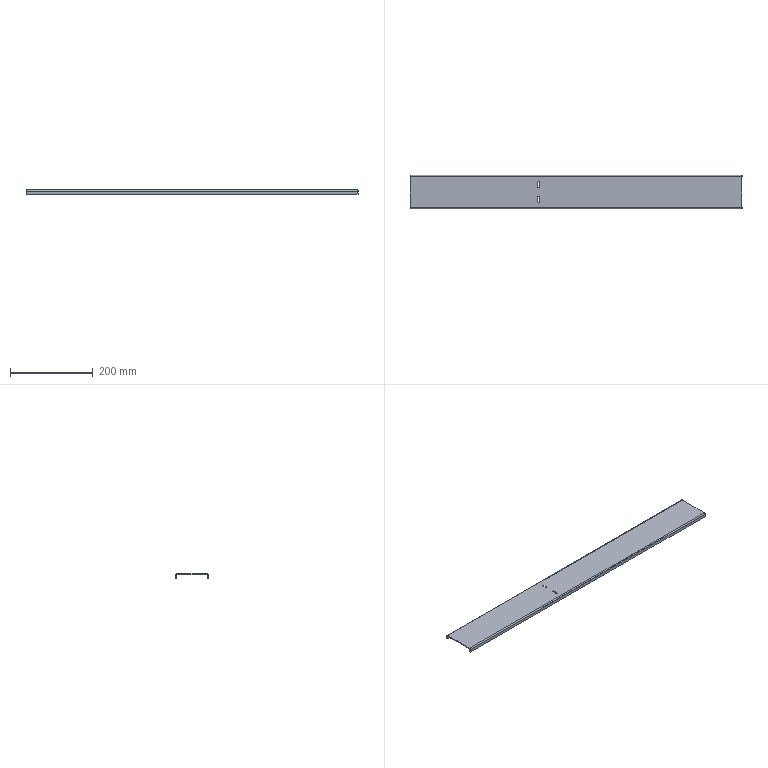Part | SolidWorks | features EdgeFlange 1, FlatPattern 1, ICE 1, SMBaseFlange 1, SheetMetal 1 | 1 solid | 30 faces | box 800 x 80 x 10 mm | volume 150971 mm3 | plane 22 | cylinder 8 | commonest cylinder face diameters 4.5 x4 1.473 x2 5.473 x2
STEP:
#1=CARTESIAN_POINT('',(-87.75,-12.5,-2.));
#2=VERTEX_POINT('',#1);
#3=CARTESIAN_POINT('',(-87.75,-22.5,-2.));
#4=VERTEX_POINT('',#3);
#5=CARTESIAN_POINT('',(-87.75,-12.5,-2.));
#6=DIRECTION('',(0.,-1.,0.));
#7=VECTOR('',#6,1000.);
#8=LINE('',#5,#7);
#9=EDGE_CURVE('',#2,#4,#8,.T.);
#10=ORIENTED_EDGE('',*,*,#9,.F.);
#11=CARTESIAN_POINT('',(-92.25,-12.5,-2.));
#12=VERTEX_POINT('',#11);
#13=CARTESIAN_POINT('',(-90.,-12.5,-2.));
#14=DIRECTION('',(0.,0.,-1.));
#15=DIRECTION('',(-1.,0.,0.));
#16=AXIS2_PLACEMENT_3D('',#13,#14,#15);
#17=CIRCLE('',#16,2.25);
#18=EDGE_CURVE('',#12,#2,#17,.T.);
#19=ORIENTED_EDGE('',*,*,#18,.F.);
#20=CARTESIAN_POINT('',(-92.25,-22.5,-2.));
#21=VERTEX_POINT('',#20);
#22=CARTESIAN_POINT('',(-92.25,-12.5,-2.));
#23=DIRECTION('',(0.,1.,0.));
#24=VECTOR('',#23,1000.);
#25=LINE('',#22,#24);
#26=EDGE_CURVE('',#21,#12,#25,.T.);
#27=ORIENTED_EDGE('',*,*,#26,.F.);
#28=CARTESIAN_POINT('',(-90.,-22.5,-2.));
#29=DIRECTION('',(0.,0.,-1.));
#30=DIRECTION('',(-1.,0.,0.));
#31=AXIS2_PLACEMENT_3D('',#28,#29,#30);
#32=CIRCLE('',#31,2.25);
#33=EDGE_CURVE('',#4,#21,#32,.T.);
#34=ORIENTED_EDGE('',*,*,#33,.F.);
#35=EDGE_LOOP('',(#10,#19,#27,#34));
#36=FACE_BOUND('',#35,.T.);
#37=CARTESIAN_POINT('',(-87.75,22.5,-2.));
#38=VERTEX_POINT('',#37);
#39=CARTESIAN_POINT('',(-87.75,12.5,-2.));
#40=VERTEX_POINT('',#39);
#41=CARTESIAN_POINT('',(-87.75,22.5,-2.));
#42=DIRECTION('',(0.,-1.,0.));
#43=VECTOR('',#42,1000.);
#44=LINE('',#41,#43);
#45=EDGE_CURVE('',#38,#40,#44,.T.);
#46=ORIENTED_EDGE('',*,*,#45,.F.);
#47=CARTESIAN_POINT('',(-92.25,22.5,-2.));
#48=VERTEX_POINT('',#47);
#49=CARTESIAN_POINT('',(-90.,22.5,-2.));
#50=DIRECTION('',(0.,0.,-1.));
#51=DIRECTION('',(-1.,0.,0.));
#52=AXIS2_PLACEMENT_3D('',#49,#50,#51);
#53=CIRCLE('',#52,2.25);
#54=EDGE_CURVE('',#48,#38,#53,.T.);
#55=ORIENTED_EDGE('',*,*,#54,.F.);
#56=CARTESIAN_POINT('',(-92.25,12.5,-2.));
#57=VERTEX_POINT('',#56);
#58=CARTESIAN_POINT('',(-92.25,22.5,-2.));
#59=DIRECTION('',(0.,1.,0.));
#60=VECTOR('',#59,1000.);
#61=LINE('',#58,#60);
#62=EDGE_CURVE('',#57,#48,#61,.T.);
#63=ORIENTED_EDGE('',*,*,#62,.F.);
#64=CARTESIAN_POINT('',(-90.,12.5,-2.));
#65=DIRECTION('',(0.,0.,-1.));
#66=DIRECTION('',(-1.,0.,0.));
#67=AXIS2_PLACEMENT_3D('',#64,#65,#66);
#68=CIRCLE('',#67,2.25);
#69=EDGE_CURVE('',#40,#57,#68,.T.);
#70=ORIENTED_EDGE('',*,*,#69,.F.);
#71=EDGE_LOOP('',(#46,#55,#63,#70));
#72=FACE_BOUND('',#71,.T.);
#73=CARTESIAN_POINT('',(-400.,-37.263,-2.));
#74=VERTEX_POINT('',#73);
#75=CARTESIAN_POINT('',(400.,-37.263,-2.));
#76=VERTEX_POINT('',#75);
#77=CARTESIAN_POINT('',(-400.,-37.263,-2.));
#78=DIRECTION('',(1.,0.,0.));
#79=VECTOR('',#78,1000.);
#80=LINE('',#77,#79);
#81=EDGE_CURVE('',#74,#76,#80,.T.);
#82=ORIENTED_EDGE('',*,*,#81,.F.);
#83=CARTESIAN_POINT('',(-400.,37.263,-2.));
#84=VERTEX_POINT('',#83);
#85=CARTESIAN_POINT('',(-400.,40.,-2.));
#86=DIRECTION('',(0.,-1.,0.));
#87=VECTOR('',#86,1000.);
#88=LINE('',#85,#87);
#89=EDGE_CURVE('',#84,#74,#88,.T.);
#90=ORIENTED_EDGE('',*,*,#89,.F.);
#91=CARTESIAN_POINT('',(400.,37.263,-2.));
#92=VERTEX_POINT('',#91);
#93=CARTESIAN_POINT('',(400.,37.263,-2.));
#94=DIRECTION('',(-1.,0.,0.));
#95=VECTOR('',#94,1000.);
#96=LINE('',#93,#95);
#97=EDGE_CURVE('',#92,#84,#96,.T.);
#98=ORIENTED_EDGE('',*,*,#97,.F.);
#99=CARTESIAN_POINT('',(400.,40.,-2.));
#100=DIRECTION('',(0.,1.,0.));
#101=VECTOR('',#100,1000.);
#102=LINE('',#99,#101);
#103=EDGE_CURVE('',#76,#92,#102,.T.);
#104=ORIENTED_EDGE('',*,*,#103,.F.);
#105=EDGE_LOOP('',(#82,#90,#98,#104));
#106=FACE_OUTER_BOUND('',#105,.T.);
#107=CARTESIAN_POINT('',(0.,0.,-2.));
#108=DIRECTION('',(0.,0.,1.));
#109=DIRECTION('',(1.,0.,0.));
#110=AXIS2_PLACEMENT_3D('',#107,#108,#109);
#111=PLANE('',#110);
#112=ADVANCED_FACE('',(#36,#72,#106),#111,.F.);
#113=CARTESIAN_POINT('',(-87.75,-12.5,0.));
#114=VERTEX_POINT('',#113);
#115=CARTESIAN_POINT('',(-92.25,-12.5,0.));
#116=VERTEX_POINT('',#115);
#117=CARTESIAN_POINT('',(-90.,-12.5,0.));
#118=DIRECTION('',(0.,0.,1.));
#119=DIRECTION('',(1.,0.,0.));
#120=AXIS2_PLACEMENT_3D('',#117,#118,#119);
#121=CIRCLE('',#120,2.25);
#122=EDGE_CURVE('',#114,#116,#121,.T.);
#123=ORIENTED_EDGE('',*,*,#122,.F.);
#124=CARTESIAN_POINT('',(-87.75,-22.5,0.));
#125=VERTEX_POINT('',#124);
#126=CARTESIAN_POINT('',(-87.75,0.,0.));
#127=DIRECTION('',(0.,1.,0.));
#128=VECTOR('',#127,1000.);
#129=LINE('',#126,#128);
#130=EDGE_CURVE('',#125,#114,#129,.T.);
#131=ORIENTED_EDGE('',*,*,#130,.F.);
#132=CARTESIAN_POINT('',(-92.25,-22.5,0.));
#133=VERTEX_POINT('',#132);
#134=CARTESIAN_POINT('',(-90.,-22.5,0.));
#135=DIRECTION('',(0.,0.,1.));
#136=DIRECTION('',(1.,0.,0.));
#137=AXIS2_PLACEMENT_3D('',#134,#135,#136);
#138=CIRCLE('',#137,2.25);
#139=EDGE_CURVE('',#133,#125,#138,.T.);
#140=ORIENTED_EDGE('',*,*,#139,.F.);
#141=CARTESIAN_POINT('',(-92.25,0.,0.));
#142=DIRECTION('',(0.,-1.,0.));
#143=VECTOR('',#142,1000.);
#144=LINE('',#141,#143);
#145=EDGE_CURVE('',#116,#133,#144,.T.);
#146=ORIENTED_EDGE('',*,*,#145,.F.);
#147=EDGE_LOOP('',(#123,#131,#140,#146));
#148=FACE_BOUND('',#147,.T.);
#149=CARTESIAN_POINT('',(-87.75,22.5,0.));
#150=VERTEX_POINT('',#149);
#151=CARTESIAN_POINT('',(-92.25,22.5,0.));
#152=VERTEX_POINT('',#151);
#153=CARTESIAN_POINT('',(-90.,22.5,0.));
#154=DIRECTION('',(0.,0.,1.));
#155=DIRECTION('',(1.,0.,0.));
#156=AXIS2_PLACEMENT_3D('',#153,#154,#155);
#157=CIRCLE('',#156,2.25);
#158=EDGE_CURVE('',#150,#152,#157,.T.);
#159=ORIENTED_EDGE('',*,*,#158,.F.);
#160=CARTESIAN_POINT('',(-87.75,12.5,0.));
#161=VERTEX_POINT('',#160);
#162=CARTESIAN_POINT('',(-87.75,0.,0.));
#163=DIRECTION('',(0.,1.,0.));
#164=VECTOR('',#163,1000.);
#165=LINE('',#162,#164);
#166=EDGE_CURVE('',#161,#150,#165,.T.);
#167=ORIENTED_EDGE('',*,*,#166,.F.);
#168=CARTESIAN_POINT('',(-92.25,12.5,0.));
#169=VERTEX_POINT('',#168);
#170=CARTESIAN_POINT('',(-90.,12.5,0.));
#171=DIRECTION('',(0.,0.,1.));
#172=DIRECTION('',(1.,0.,0.));
#173=AXIS2_PLACEMENT_3D('',#170,#171,#172);
#174=CIRCLE('',#173,2.25);
#175=EDGE_CURVE('',#169,#161,#174,.T.);
#176=ORIENTED_EDGE('',*,*,#175,.F.);
#177=CARTESIAN_POINT('',(-92.25,0.,0.));
#178=DIRECTION('',(0.,-1.,0.));
#179=VECTOR('',#178,1000.);
#180=LINE('',#177,#179);
#181=EDGE_CURVE('',#152,#169,#180,.T.);
#182=ORIENTED_EDGE('',*,*,#181,.F.);
#183=EDGE_LOOP('',(#159,#167,#176,#182));
#184=FACE_BOUND('',#183,.T.);
#185=CARTESIAN_POINT('',(-400.,37.263,0.));
#186=VERTEX_POINT('',#185);
#187=CARTESIAN_POINT('',(-400.,-37.263,0.));
#188=VERTEX_POINT('',#187);
#189=CARTESIAN_POINT('',(-400.,40.,0.));
#190=DIRECTION('',(0.,-1.,0.));
#191=VECTOR('',#190,1000.);
#192=LINE('',#189,#191);
#193=EDGE_CURVE('',#186,#188,#192,.T.);
#194=ORIENTED_EDGE('',*,*,#193,.T.);
#195=CARTESIAN_POINT('',(400.,-37.263,0.));
#196=VERTEX_POINT('',#195);
#197=CARTESIAN_POINT('',(-400.,-37.263,0.));
#198=DIRECTION('',(1.,0.,0.));
#199=VECTOR('',#198,1000.);
#200=LINE('',#197,#199);
#201=EDGE_CURVE('',#188,#196,#200,.T.);
#202=ORIENTED_EDGE('',*,*,#201,.T.);
#203=CARTESIAN_POINT('',(400.,37.263,0.));
#204=VERTEX_POINT('',#203);
#205=CARTESIAN_POINT('',(400.,40.,0.));
#206=DIRECTION('',(0.,1.,0.));
#207=VECTOR('',#206,1000.);
#208=LINE('',#205,#207);
#209=EDGE_CURVE('',#196,#204,#208,.T.);
#210=ORIENTED_EDGE('',*,*,#209,.T.);
#211=CARTESIAN_POINT('',(400.,37.263,0.));
#212=DIRECTION('',(-1.,0.,0.));
#213=VECTOR('',#212,1000.);
#214=LINE('',#211,#213);
#215=EDGE_CURVE('',#204,#186,#214,.T.);
#216=ORIENTED_EDGE('',*,*,#215,.T.);
#217=EDGE_LOOP('',(#194,#202,#210,#216));
#218=FACE_OUTER_BOUND('',#217,.T.);
#219=CARTESIAN_POINT('',(0.,0.,0.));
#220=DIRECTION('',(0.,0.,1.));
#221=DIRECTION('',(1.,0.,0.));
#222=AXIS2_PLACEMENT_3D('',#219,#220,#221);
#223=PLANE('',#222);
#224=ADVANCED_FACE('',(#148,#184,#218),#223,.T.);
#225=ORIENTED_EDGE('',*,*,#89,.T.);
#226=CARTESIAN_POINT('',(-400.,-37.263,-2.));
#227=DIRECTION('',(0.,0.,1.));
#228=VECTOR('',#227,1000.);
#229=LINE('',#226,#228);
#230=EDGE_CURVE('',#74,#188,#229,.T.);
#231=ORIENTED_EDGE('',*,*,#230,.T.);
#232=ORIENTED_EDGE('',*,*,#193,.F.);
#233=CARTESIAN_POINT('',(-400.,37.263,-2.));
#234=DIRECTION('',(0.,0.,1.));
#235=VECTOR('',#234,1000.);
#236=LINE('',#233,#235);
#237=EDGE_CURVE('',#84,#186,#236,.T.);
#238=ORIENTED_EDGE('',*,*,#237,.F.);
#239=EDGE_LOOP('',(#225,#231,#232,#238));
#240=FACE_OUTER_BOUND('',#239,.T.);
#241=CARTESIAN_POINT('',(-400.,40.,-2.));
#242=DIRECTION('',(-1.,0.,0.));
#243=DIRECTION('',(0.,0.,1.));
#244=AXIS2_PLACEMENT_3D('',#241,#242,#243);
#245=PLANE('',#244);
#246=ADVANCED_FACE('',(#240),#245,.T.);
#247=CARTESIAN_POINT('',(400.,-37.263,-2.));
#248=DIRECTION('',(0.,0.,1.));
#249=VECTOR('',#248,1000.);
#250=LINE('',#247,#249);
#251=EDGE_CURVE('',#76,#196,#250,.T.);
#252=ORIENTED_EDGE('',*,*,#251,.F.);
#253=ORIENTED_EDGE('',*,*,#103,.T.);
#254=CARTESIAN_POINT('',(400.,37.263,-2.));
#255=DIRECTION('',(0.,0.,1.));
#256=VECTOR('',#255,1000.);
#257=LINE('',#254,#256);
#258=EDGE_CURVE('',#92,#204,#257,.T.);
#259=ORIENTED_EDGE('',*,*,#258,.T.);
#260=ORIENTED_EDGE('',*,*,#209,.F.);
#261=EDGE_LOOP('',(#252,#253,#259,#260));
#262=FACE_OUTER_BOUND('',#261,.T.);
#263=CARTESIAN_POINT('',(400.,40.,-2.));
#264=DIRECTION('',(1.,0.,0.));
#265=DIRECTION('',(0.,0.,-1.));
#266=AXIS2_PLACEMENT_3D('',#263,#264,#265);
#267=PLANE('',#266);
#268=ADVANCED_FACE('',(#262),#267,.T.);
#269=CARTESIAN_POINT('',(-400.,38.,-2.737));
#270=VERTEX_POINT('',#269);
#271=CARTESIAN_POINT('',(-400.,40.,-2.737));
#272=VERTEX_POINT('',#271);
#273=CARTESIAN_POINT('',(-400.,40.,-2.737));
#274=DIRECTION('',(0.,1.,0.));
#275=VECTOR('',#274,1000.);
#276=LINE('',#273,#275);
#277=EDGE_CURVE('',#270,#272,#276,.T.);
#278=ORIENTED_EDGE('',*,*,#277,.F.);
#279=CARTESIAN_POINT('',(-400.,37.263,-2.737));
#280=DIRECTION('',(-1.,0.,0.));
#281=DIRECTION('',(0.,0.,-1.));
#282=AXIS2_PLACEMENT_3D('',#279,#280,#281);
#283=CIRCLE('',#282,0.7366);
#284=EDGE_CURVE('',#84,#270,#283,.T.);
#285=ORIENTED_EDGE('',*,*,#284,.F.);
#286=ORIENTED_EDGE('',*,*,#237,.T.);
#287=CARTESIAN_POINT('',(-400.,37.263,-2.737));
#288=DIRECTION('',(-1.,0.,0.));
#289=DIRECTION('',(0.,0.,-1.));
#290=AXIS2_PLACEMENT_3D('',#287,#288,#289);
#291=CIRCLE('',#290,2.737);
#292=EDGE_CURVE('',#186,#272,#291,.T.);
#293=ORIENTED_EDGE('',*,*,#292,.T.);
#294=EDGE_LOOP('',(#278,#285,#286,#293));
#295=FACE_OUTER_BOUND('',#294,.T.);
#296=CARTESIAN_POINT('',(-400.,37.263,-2.737));
#297=DIRECTION('',(-1.,0.,0.));
#298=DIRECTION('',(0.,0.,1.));
#299=AXIS2_PLACEMENT_3D('',#296,#297,#298);
#300=PLANE('',#299);
#301=ADVANCED_FACE('',(#295),#300,.T.);
#302=CARTESIAN_POINT('',(400.,38.,-2.737));
#303=VERTEX_POINT('',#302);
#304=CARTESIAN_POINT('',(400.,37.263,-2.737));
#305=DIRECTION('',(1.,0.,0.));
#306=DIRECTION('',(0.,0.,-1.));
#307=AXIS2_PLACEMENT_3D('',#304,#305,#306);
#308=CIRCLE('',#307,0.7366);
#309=EDGE_CURVE('',#303,#92,#308,.T.);
#310=ORIENTED_EDGE('',*,*,#309,.F.);
#311=CARTESIAN_POINT('',(400.,40.,-2.737));
#312=VERTEX_POINT('',#311);
#313=CARTESIAN_POINT('',(400.,38.,-2.737));
#314=DIRECTION('',(0.,1.,0.));
#315=VECTOR('',#314,1000.);
#316=LINE('',#313,#315);
#317=EDGE_CURVE('',#303,#312,#316,.T.);
#318=ORIENTED_EDGE('',*,*,#317,.T.);
#319=CARTESIAN_POINT('',(400.,37.263,-2.737));
#320=DIRECTION('',(1.,0.,0.));
#321=DIRECTION('',(0.,0.,-1.));
#322=AXIS2_PLACEMENT_3D('',#319,#320,#321);
#323=CIRCLE('',#322,2.737);
#324=EDGE_CURVE('',#312,#204,#323,.T.);
#325=ORIENTED_EDGE('',*,*,#324,.T.);
#326=ORIENTED_EDGE('',*,*,#258,.F.);
#327=EDGE_LOOP('',(#310,#318,#325,#326));
#328=FACE_OUTER_BOUND('',#327,.T.);
#329=CARTESIAN_POINT('',(400.,37.263,-2.737));
#330=DIRECTION('',(-1.,0.,0.));
#331=DIRECTION('',(0.,0.,1.));
#332=AXIS2_PLACEMENT_3D('',#329,#330,#331);
#333=PLANE('',#332);
#334=ADVANCED_FACE('',(#328),#333,.F.);
#335=ORIENTED_EDGE('',*,*,#215,.F.);
#336=ORIENTED_EDGE('',*,*,#324,.F.);
#337=CARTESIAN_POINT('',(0.,40.,-2.737));
#338=DIRECTION('',(1.,0.,0.));
#339=VECTOR('',#338,1000.);
#340=LINE('',#337,#339);
#341=EDGE_CURVE('',#272,#312,#340,.T.);
#342=ORIENTED_EDGE('',*,*,#341,.F.);
#343=ORIENTED_EDGE('',*,*,#292,.F.);
#344=EDGE_LOOP('',(#335,#336,#342,#343));
#345=FACE_OUTER_BOUND('',#344,.T.);
#346=CARTESIAN_POINT('',(400.,37.263,-2.737));
#347=DIRECTION('',(1.,0.,0.));
#348=DIRECTION('',(0.,1.,0.));
#349=AXIS2_PLACEMENT_3D('',#346,#347,#348);
#350=CYLINDRICAL_SURFACE('',#349,2.737);
#351=ADVANCED_FACE('',(#345),#350,.T.);
#352=ORIENTED_EDGE('',*,*,#97,.T.);
#353=ORIENTED_EDGE('',*,*,#284,.T.);
#354=CARTESIAN_POINT('',(-400.,38.,-2.737));
#355=DIRECTION('',(1.,0.,0.));
#356=VECTOR('',#355,1000.);
#357=LINE('',#354,#356);
#358=EDGE_CURVE('',#270,#303,#357,.T.);
#359=ORIENTED_EDGE('',*,*,#358,.T.);
#360=ORIENTED_EDGE('',*,*,#309,.T.);
#361=EDGE_LOOP('',(#352,#353,#359,#360));
#362=FACE_OUTER_BOUND('',#361,.T.);
#363=CARTESIAN_POINT('',(400.,37.263,-2.737));
#364=DIRECTION('',(1.,0.,0.));
#365=DIRECTION('',(0.,1.,0.));
#366=AXIS2_PLACEMENT_3D('',#363,#364,#365);
#367=CYLINDRICAL_SURFACE('',#366,0.7366);
#368=ADVANCED_FACE('',(#362),#367,.F.);
#369=CARTESIAN_POINT('',(400.,40.,-10.));
#370=VERTEX_POINT('',#369);
#371=CARTESIAN_POINT('',(400.,40.,-2.));
#372=DIRECTION('',(0.,0.,1.));
#373=VECTOR('',#372,1000.);
#374=LINE('',#371,#373);
#375=EDGE_CURVE('',#370,#312,#374,.T.);
#376=ORIENTED_EDGE('',*,*,#375,.T.);
#377=ORIENTED_EDGE('',*,*,#317,.F.);
#378=CARTESIAN_POINT('',(400.,38.,-10.));
#379=VERTEX_POINT('',#378);
#380=CARTESIAN_POINT('',(400.,38.,0.));
#381=DIRECTION('',(0.,0.,1.));
#382=VECTOR('',#381,1000.);
#383=LINE('',#380,#382);
#384=EDGE_CURVE('',#379,#303,#383,.T.);
#385=ORIENTED_EDGE('',*,*,#384,.F.);
#386=CARTESIAN_POINT('',(400.,40.,-10.));
#387=DIRECTION('',(0.,-1.,0.));
#388=VECTOR('',#387,1000.);
#389=LINE('',#386,#388);
#390=EDGE_CURVE('',#370,#379,#389,.T.);
#391=ORIENTED_EDGE('',*,*,#390,.F.);
#392=EDGE_LOOP('',(#376,#377,#385,#391));
#393=FACE_OUTER_BOUND('',#392,.T.);
#394=CARTESIAN_POINT('',(400.,40.,-2.));
#395=DIRECTION('',(1.,0.,0.));
#396=DIRECTION('',(0.,0.,-1.));
#397=AXIS2_PLACEMENT_3D('',#394,#395,#396);
#398=PLANE('',#397);
#399=ADVANCED_FACE('',(#393),#398,.T.);
#400=CARTESIAN_POINT('',(-400.,38.,-10.));
#401=VERTEX_POINT('',#400);
#402=CARTESIAN_POINT('',(-400.,38.,0.));
#403=DIRECTION('',(0.,0.,-1.));
#404=VECTOR('',#403,1000.);
#405=LINE('',#402,#404);
#406=EDGE_CURVE('',#270,#401,#405,.T.);
#407=ORIENTED_EDGE('',*,*,#406,.F.);
#408=ORIENTED_EDGE('',*,*,#277,.T.);
#409=CARTESIAN_POINT('',(-400.,40.,-10.));
#410=VERTEX_POINT('',#409);
#411=CARTESIAN_POINT('',(-400.,40.,-10.));
#412=DIRECTION('',(0.,0.,-1.));
#413=VECTOR('',#412,1000.);
#414=LINE('',#411,#413);
#415=EDGE_CURVE('',#272,#410,#414,.T.);
#416=ORIENTED_EDGE('',*,*,#415,.T.);
#417=CARTESIAN_POINT('',(-400.,40.,-10.));
#418=DIRECTION('',(0.,-1.,0.));
#419=VECTOR('',#418,1000.);
#420=LINE('',#417,#419);
#421=EDGE_CURVE('',#410,#401,#420,.T.);
#422=ORIENTED_EDGE('',*,*,#421,.T.);
#423=EDGE_LOOP('',(#407,#408,#416,#422));
#424=FACE_OUTER_BOUND('',#423,.T.);
#425=CARTESIAN_POINT('',(-400.,40.,-10.));
#426=DIRECTION('',(-1.,0.,0.));
#427=DIRECTION('',(0.,0.,1.));
#428=AXIS2_PLACEMENT_3D('',#425,#426,#427);
#429=PLANE('',#428);
#430=ADVANCED_FACE('',(#424),#429,.T.);
#431=ORIENTED_EDGE('',*,*,#415,.F.);
#432=ORIENTED_EDGE('',*,*,#341,.T.);
#433=ORIENTED_EDGE('',*,*,#375,.F.);
#434=CARTESIAN_POINT('',(400.,40.,-10.));
#435=DIRECTION('',(1.,0.,0.));
#436=VECTOR('',#435,1000.);
#437=LINE('',#434,#436);
#438=EDGE_CURVE('',#410,#370,#437,.T.);
#439=ORIENTED_EDGE('',*,*,#438,.F.);
#440=EDGE_LOOP('',(#431,#432,#433,#439));
#441=FACE_OUTER_BOUND('',#440,.T.);
#442=CARTESIAN_POINT('',(0.,40.,0.));
#443=DIRECTION('',(0.,1.,0.));
#444=DIRECTION('',(0.,0.,1.));
#445=AXIS2_PLACEMENT_3D('',#442,#443,#444);
#446=PLANE('',#445);
#447=ADVANCED_FACE('',(#441),#446,.T.);
#448=ORIENTED_EDGE('',*,*,#358,.F.);
#449=ORIENTED_EDGE('',*,*,#406,.T.);
#450=CARTESIAN_POINT('',(0.,38.,-10.));
#451=DIRECTION('',(1.,0.,0.));
#452=VECTOR('',#451,1000.);
#453=LINE('',#450,#452);
#454=EDGE_CURVE('',#401,#379,#453,.T.);
#455=ORIENTED_EDGE('',*,*,#454,.T.);
#456=ORIENTED_EDGE('',*,*,#384,.T.);
#457=EDGE_LOOP('',(#448,#449,#455,#456));
#458=FACE_OUTER_BOUND('',#457,.T.);
#459=CARTESIAN_POINT('',(0.,38.,0.));
#460=DIRECTION('',(0.,1.,0.));
#461=DIRECTION('',(0.,0.,1.));
#462=AXIS2_PLACEMENT_3D('',#459,#460,#461);
#463=PLANE('',#462);
#464=ADVANCED_FACE('',(#458),#463,.F.);
#465=ORIENTED_EDGE('',*,*,#454,.F.);
#466=ORIENTED_EDGE('',*,*,#421,.F.);
#467=ORIENTED_EDGE('',*,*,#438,.T.);
#468=ORIENTED_EDGE('',*,*,#390,.T.);
#469=EDGE_LOOP('',(#465,#466,#467,#468));
#470=FACE_OUTER_BOUND('',#469,.T.);
#471=CARTESIAN_POINT('',(400.,40.,-10.));
#472=DIRECTION('',(0.,0.,-1.));
#473=DIRECTION('',(0.,1.,0.));
#474=AXIS2_PLACEMENT_3D('',#471,#472,#473);
#475=PLANE('',#474);
#476=ADVANCED_FACE('',(#470),#475,.T.);
#477=CARTESIAN_POINT('',(400.,-38.,-2.737));
#478=VERTEX_POINT('',#477);
#479=CARTESIAN_POINT('',(400.,-40.,-2.737));
#480=VERTEX_POINT('',#479);
#481=CARTESIAN_POINT('',(400.,-40.,-2.737));
#482=DIRECTION('',(0.,-1.,0.));
#483=VECTOR('',#482,1000.);
#484=LINE('',#481,#483);
#485=EDGE_CURVE('',#478,#480,#484,.T.);
#486=ORIENTED_EDGE('',*,*,#485,.F.);
#487=CARTESIAN_POINT('',(400.,-37.263,-2.737));
#488=DIRECTION('',(1.,0.,0.));
#489=DIRECTION('',(0.,0.,1.));
#490=AXIS2_PLACEMENT_3D('',#487,#488,#489);
#491=CIRCLE('',#490,0.7366);
#492=EDGE_CURVE('',#76,#478,#491,.T.);
#493=ORIENTED_EDGE('',*,*,#492,.F.);
#494=ORIENTED_EDGE('',*,*,#251,.T.);
#495=CARTESIAN_POINT('',(400.,-37.263,-2.737));
#496=DIRECTION('',(1.,0.,0.));
#497=DIRECTION('',(0.,0.,1.));
#498=AXIS2_PLACEMENT_3D('',#495,#496,#497);
#499=CIRCLE('',#498,2.737);
#500=EDGE_CURVE('',#196,#480,#499,.T.);
#501=ORIENTED_EDGE('',*,*,#500,.T.);
#502=EDGE_LOOP('',(#486,#493,#494,#501));
#503=FACE_OUTER_BOUND('',#502,.T.);
#504=CARTESIAN_POINT('',(400.,-37.263,-2.737));
#505=DIRECTION('',(1.,0.,0.));
#506=DIRECTION('',(0.,0.,-1.));
#507=AXIS2_PLACEMENT_3D('',#504,#505,#506);
#508=PLANE('',#507);
#509=ADVANCED_FACE('',(#503),#508,.T.);
#510=CARTESIAN_POINT('',(-400.,-38.,-2.737));
#511=VERTEX_POINT('',#510);
#512=CARTESIAN_POINT('',(-400.,-37.263,-2.737));
#513=DIRECTION('',(-1.,0.,0.));
#514=DIRECTION('',(0.,0.,1.));
#515=AXIS2_PLACEMENT_3D('',#512,#513,#514);
#516=CIRCLE('',#515,0.7366);
#517=EDGE_CURVE('',#511,#74,#516,.T.);
#518=ORIENTED_EDGE('',*,*,#517,.F.);
#519=CARTESIAN_POINT('',(-400.,-40.,-2.737));
#520=VERTEX_POINT('',#519);
#521=CARTESIAN_POINT('',(-400.,-38.,-2.737));
#522=DIRECTION('',(0.,-1.,0.));
#523=VECTOR('',#522,1000.);
#524=LINE('',#521,#523);
#525=EDGE_CURVE('',#511,#520,#524,.T.);
#526=ORIENTED_EDGE('',*,*,#525,.T.);
#527=CARTESIAN_POINT('',(-400.,-37.263,-2.737));
#528=DIRECTION('',(-1.,0.,0.));
#529=DIRECTION('',(0.,0.,1.));
#530=AXIS2_PLACEMENT_3D('',#527,#528,#529);
#531=CIRCLE('',#530,2.737);
#532=EDGE_CURVE('',#520,#188,#531,.T.);
#533=ORIENTED_EDGE('',*,*,#532,.T.);
#534=ORIENTED_EDGE('',*,*,#230,.F.);
#535=EDGE_LOOP('',(#518,#526,#533,#534));
#536=FACE_OUTER_BOUND('',#535,.T.);
#537=CARTESIAN_POINT('',(-400.,-37.263,-2.737));
#538=DIRECTION('',(1.,0.,0.));
#539=DIRECTION('',(0.,0.,-1.));
#540=AXIS2_PLACEMENT_3D('',#537,#538,#539);
#541=PLANE('',#540);
#542=ADVANCED_FACE('',(#536),#541,.F.);
#543=ORIENTED_EDGE('',*,*,#201,.F.);
#544=ORIENTED_EDGE('',*,*,#532,.F.);
#545=CARTESIAN_POINT('',(400.,-40.,-2.737));
#546=DIRECTION('',(1.,0.,0.));
#547=VECTOR('',#546,1000.);
#548=LINE('',#545,#547);
#549=EDGE_CURVE('',#520,#480,#548,.T.);
#550=ORIENTED_EDGE('',*,*,#549,.T.);
#551=ORIENTED_EDGE('',*,*,#500,.F.);
#552=EDGE_LOOP('',(#543,#544,#550,#551));
#553=FACE_OUTER_BOUND('',#552,.T.);
#554=CARTESIAN_POINT('',(-400.,-37.263,-2.737));
#555=DIRECTION('',(-1.,0.,0.));
#556=DIRECTION('',(0.,-1.,0.));
#557=AXIS2_PLACEMENT_3D('',#554,#555,#556);
#558=CYLINDRICAL_SURFACE('',#557,2.737);
#559=ADVANCED_FACE('',(#553),#558,.T.);
#560=ORIENTED_EDGE('',*,*,#81,.T.);
#561=ORIENTED_EDGE('',*,*,#492,.T.);
#562=CARTESIAN_POINT('',(400.,-38.,-2.737));
#563=DIRECTION('',(-1.,0.,0.));
#564=VECTOR('',#563,1000.);
#565=LINE('',#562,#564);
#566=EDGE_CURVE('',#478,#511,#565,.T.);
#567=ORIENTED_EDGE('',*,*,#566,.T.);
#568=ORIENTED_EDGE('',*,*,#517,.T.);
#569=EDGE_LOOP('',(#560,#561,#567,#568));
#570=FACE_OUTER_BOUND('',#569,.T.);
#571=CARTESIAN_POINT('',(-400.,-37.263,-2.737));
#572=DIRECTION('',(-1.,0.,0.));
#573=DIRECTION('',(0.,-1.,0.));
#574=AXIS2_PLACEMENT_3D('',#571,#572,#573);
#575=CYLINDRICAL_SURFACE('',#574,0.7366);
#576=ADVANCED_FACE('',(#570),#575,.F.);
#577=CARTESIAN_POINT('',(400.,-38.,-10.));
#578=VERTEX_POINT('',#577);
#579=CARTESIAN_POINT('',(400.,-38.,0.));
#580=DIRECTION('',(0.,0.,-1.));
#581=VECTOR('',#580,1000.);
#582=LINE('',#579,#581);
#583=EDGE_CURVE('',#478,#578,#582,.T.);
#584=ORIENTED_EDGE('',*,*,#583,.F.);
#585=ORIENTED_EDGE('',*,*,#485,.T.);
#586=CARTESIAN_POINT('',(400.,-40.,-10.));
#587=VERTEX_POINT('',#586);
#588=CARTESIAN_POINT('',(400.,-40.,-2.));
#589=DIRECTION('',(0.,0.,-1.));
#590=VECTOR('',#589,1000.);
#591=LINE('',#588,#590);
#592=EDGE_CURVE('',#480,#587,#591,.T.);
#593=ORIENTED_EDGE('',*,*,#592,.T.);
#594=CARTESIAN_POINT('',(400.,-40.,-10.));
#595=DIRECTION('',(0.,1.,0.));
#596=VECTOR('',#595,1000.);
#597=LINE('',#594,#596);
#598=EDGE_CURVE('',#587,#578,#597,.T.);
#599=ORIENTED_EDGE('',*,*,#598,.T.);
#600=EDGE_LOOP('',(#584,#585,#593,#599));
#601=FACE_OUTER_BOUND('',#600,.T.);
#602=CARTESIAN_POINT('',(400.,-40.,-2.));
#603=DIRECTION('',(1.,0.,0.));
#604=DIRECTION('',(0.,0.,-1.));
#605=AXIS2_PLACEMENT_3D('',#602,#603,#604);
#606=PLANE('',#605);
#607=ADVANCED_FACE('',(#601),#606,.T.);
#608=CARTESIAN_POINT('',(-400.,-40.,-10.));
#609=VERTEX_POINT('',#608);
#610=CARTESIAN_POINT('',(-400.,-40.,-10.));
#611=DIRECTION('',(0.,0.,1.));
#612=VECTOR('',#611,1000.);
#613=LINE('',#610,#612);
#614=EDGE_CURVE('',#609,#520,#613,.T.);
#615=ORIENTED_EDGE('',*,*,#614,.T.);
#616=ORIENTED_EDGE('',*,*,#525,.F.);
#617=CARTESIAN_POINT('',(-400.,-38.,-10.));
#618=VERTEX_POINT('',#617);
#619=CARTESIAN_POINT('',(-400.,-38.,0.));
#620=DIRECTION('',(0.,0.,1.));
#621=VECTOR('',#620,1000.);
#622=LINE('',#619,#621);
#623=EDGE_CURVE('',#618,#511,#622,.T.);
#624=ORIENTED_EDGE('',*,*,#623,.F.);
#625=CARTESIAN_POINT('',(-400.,-40.,-10.));
#626=DIRECTION('',(0.,1.,0.));
#627=VECTOR('',#626,1000.);
#628=LINE('',#625,#627);
#629=EDGE_CURVE('',#609,#618,#628,.T.);
#630=ORIENTED_EDGE('',*,*,#629,.F.);
#631=EDGE_LOOP('',(#615,#616,#624,#630));
#632=FACE_OUTER_BOUND('',#631,.T.);
#633=CARTESIAN_POINT('',(-400.,-40.,-10.));
#634=DIRECTION('',(-1.,0.,0.));
#635=DIRECTION('',(0.,0.,1.));
#636=AXIS2_PLACEMENT_3D('',#633,#634,#635);
#637=PLANE('',#636);
#638=ADVANCED_FACE('',(#632),#637,.T.);
#639=ORIENTED_EDGE('',*,*,#549,.F.);
#640=ORIENTED_EDGE('',*,*,#614,.F.);
#641=CARTESIAN_POINT('',(400.,-40.,-10.));
#642=DIRECTION('',(-1.,0.,0.));
#643=VECTOR('',#642,1000.);
#644=LINE('',#641,#643);
#645=EDGE_CURVE('',#587,#609,#644,.T.);
#646=ORIENTED_EDGE('',*,*,#645,.F.);
#647=ORIENTED_EDGE('',*,*,#592,.F.);
#648=EDGE_LOOP('',(#639,#640,#646,#647));
#649=FACE_OUTER_BOUND('',#648,.T.);
#650=CARTESIAN_POINT('',(0.,-40.,0.));
#651=DIRECTION('',(0.,1.,0.));
#652=DIRECTION('',(0.,0.,1.));
#653=AXIS2_PLACEMENT_3D('',#650,#651,#652);
#654=PLANE('',#653);
#655=ADVANCED_FACE('',(#649),#654,.F.);
#656=ORIENTED_EDGE('',*,*,#623,.T.);
#657=ORIENTED_EDGE('',*,*,#566,.F.);
#658=ORIENTED_EDGE('',*,*,#583,.T.);
#659=CARTESIAN_POINT('',(0.,-38.,-10.));
#660=DIRECTION('',(-1.,0.,0.));
#661=VECTOR('',#660,1000.);
#662=LINE('',#659,#661);
#663=EDGE_CURVE('',#578,#618,#662,.T.);
#664=ORIENTED_EDGE('',*,*,#663,.T.);
#665=EDGE_LOOP('',(#656,#657,#658,#664));
#666=FACE_OUTER_BOUND('',#665,.T.);
#667=CARTESIAN_POINT('',(0.,-38.,0.));
#668=DIRECTION('',(0.,1.,0.));
#669=DIRECTION('',(0.,0.,1.));
#670=AXIS2_PLACEMENT_3D('',#667,#668,#669);
#671=PLANE('',#670);
#672=ADVANCED_FACE('',(#666),#671,.T.);
#673=ORIENTED_EDGE('',*,*,#663,.F.);
#674=ORIENTED_EDGE('',*,*,#598,.F.);
#675=ORIENTED_EDGE('',*,*,#645,.T.);
#676=ORIENTED_EDGE('',*,*,#629,.T.);
#677=EDGE_LOOP('',(#673,#674,#675,#676));
#678=FACE_OUTER_BOUND('',#677,.T.);
#679=CARTESIAN_POINT('',(400.,-40.,-10.));
#680=DIRECTION('',(0.,0.,-1.));
#681=DIRECTION('',(0.,1.,0.));
#682=AXIS2_PLACEMENT_3D('',#679,#680,#681);
#683=PLANE('',#682);
#684=ADVANCED_FACE('',(#678),#683,.T.);
#685=ORIENTED_EDGE('',*,*,#158,.T.);
#686=CARTESIAN_POINT('',(-92.25,22.5,8.));
#687=DIRECTION('',(0.,0.,-1.));
#688=VECTOR('',#687,1000.);
#689=LINE('',#686,#688);
#690=EDGE_CURVE('',#152,#48,#689,.T.);
#691=ORIENTED_EDGE('',*,*,#690,.T.);
#692=ORIENTED_EDGE('',*,*,#54,.T.);
#693=CARTESIAN_POINT('',(-87.75,22.5,8.));
#694=DIRECTION('',(0.,0.,-1.));
#695=VECTOR('',#694,1000.);
#696=LINE('',#693,#695);
#697=EDGE_CURVE('',#150,#38,#696,.T.);
#698=ORIENTED_EDGE('',*,*,#697,.F.);
#699=EDGE_LOOP('',(#685,#691,#692,#698));
#700=FACE_OUTER_BOUND('',#699,.T.);
#701=CARTESIAN_POINT('',(-90.,22.5,8.));
#702=DIRECTION('',(0.,0.,-1.));
#703=DIRECTION('',(-1.,0.,0.));
#704=AXIS2_PLACEMENT_3D('',#701,#702,#703);
#705=CYLINDRICAL_SURFACE('',#704,2.25);
#706=ADVANCED_FACE('',(#700),#705,.F.);
#707=ORIENTED_EDGE('',*,*,#181,.T.);
#708=CARTESIAN_POINT('',(-92.25,12.5,8.));
#709=DIRECTION('',(0.,0.,-1.));
#710=VECTOR('',#709,1000.);
#711=LINE('',#708,#710);
#712=EDGE_CURVE('',#169,#57,#711,.T.);
#713=ORIENTED_EDGE('',*,*,#712,.T.);
#714=ORIENTED_EDGE('',*,*,#62,.T.);
#715=ORIENTED_EDGE('',*,*,#690,.F.);
#716=EDGE_LOOP('',(#707,#713,#714,#715));
#717=FACE_OUTER_BOUND('',#716,.T.);
#718=CARTESIAN_POINT('',(-92.25,22.5,8.));
#719=DIRECTION('',(-1.,0.,0.));
#720=DIRECTION('',(0.,0.,1.));
#721=AXIS2_PLACEMENT_3D('',#718,#719,#720);
#722=PLANE('',#721);
#723=ADVANCED_FACE('',(#717),#722,.F.);
#724=ORIENTED_EDGE('',*,*,#175,.T.);
#725=CARTESIAN_POINT('',(-87.75,12.5,8.));
#726=DIRECTION('',(0.,0.,-1.));
#727=VECTOR('',#726,1000.);
#728=LINE('',#725,#727);
#729=EDGE_CURVE('',#161,#40,#728,.T.);
#730=ORIENTED_EDGE('',*,*,#729,.T.);
#731=ORIENTED_EDGE('',*,*,#69,.T.);
#732=ORIENTED_EDGE('',*,*,#712,.F.);
#733=EDGE_LOOP('',(#724,#730,#731,#732));
#734=FACE_OUTER_BOUND('',#733,.T.);
#735=CARTESIAN_POINT('',(-90.,12.5,8.));
#736=DIRECTION('',(0.,0.,-1.));
#737=DIRECTION('',(-1.,0.,0.));
#738=AXIS2_PLACEMENT_3D('',#735,#736,#737);
#739=CYLINDRICAL_SURFACE('',#738,2.25);
#740=ADVANCED_FACE('',(#734),#739,.F.);
#741=ORIENTED_EDGE('',*,*,#166,.T.);
#742=ORIENTED_EDGE('',*,*,#697,.T.);
#743=ORIENTED_EDGE('',*,*,#45,.T.);
#744=ORIENTED_EDGE('',*,*,#729,.F.);
#745=EDGE_LOOP('',(#741,#742,#743,#744));
#746=FACE_OUTER_BOUND('',#745,.T.);
#747=CARTESIAN_POINT('',(-87.75,22.5,8.));
#748=DIRECTION('',(1.,0.,0.));
#749=DIRECTION('',(0.,0.,-1.));
#750=AXIS2_PLACEMENT_3D('',#747,#748,#749);
#751=PLANE('',#750);
#752=ADVANCED_FACE('',(#746),#751,.F.);
#753=ORIENTED_EDGE('',*,*,#122,.T.);
#754=CARTESIAN_POINT('',(-92.25,-12.5,8.));
#755=DIRECTION('',(0.,0.,-1.));
#756=VECTOR('',#755,1000.);
#757=LINE('',#754,#756);
#758=EDGE_CURVE('',#116,#12,#757,.T.);
#759=ORIENTED_EDGE('',*,*,#758,.T.);
#760=ORIENTED_EDGE('',*,*,#18,.T.);
#761=CARTESIAN_POINT('',(-87.75,-12.5,8.));
#762=DIRECTION('',(0.,0.,-1.));
#763=VECTOR('',#762,1000.);
#764=LINE('',#761,#763);
#765=EDGE_CURVE('',#114,#2,#764,.T.);
#766=ORIENTED_EDGE('',*,*,#765,.F.);
#767=EDGE_LOOP('',(#753,#759,#760,#766));
#768=FACE_OUTER_BOUND('',#767,.T.);
#769=CARTESIAN_POINT('',(-90.,-12.5,8.));
#770=DIRECTION('',(0.,0.,-1.));
#771=DIRECTION('',(-1.,0.,0.));
#772=AXIS2_PLACEMENT_3D('',#769,#770,#771);
#773=CYLINDRICAL_SURFACE('',#772,2.25);
#774=ADVANCED_FACE('',(#768),#773,.F.);
#775=ORIENTED_EDGE('',*,*,#145,.T.);
#776=CARTESIAN_POINT('',(-92.25,-22.5,8.));
#777=DIRECTION('',(0.,0.,-1.));
#778=VECTOR('',#777,1000.);
#779=LINE('',#776,#778);
#780=EDGE_CURVE('',#133,#21,#779,.T.);
#781=ORIENTED_EDGE('',*,*,#780,.T.);
#782=ORIENTED_EDGE('',*,*,#26,.T.);
#783=ORIENTED_EDGE('',*,*,#758,.F.);
#784=EDGE_LOOP('',(#775,#781,#782,#783));
#785=FACE_OUTER_BOUND('',#784,.T.);
#786=CARTESIAN_POINT('',(-92.25,-12.5,8.));
#787=DIRECTION('',(-1.,0.,0.));
#788=DIRECTION('',(0.,0.,1.));
#789=AXIS2_PLACEMENT_3D('',#786,#787,#788);
#790=PLANE('',#789);
#791=ADVANCED_FACE('',(#785),#790,.F.);
#792=ORIENTED_EDGE('',*,*,#139,.T.);
#793=CARTESIAN_POINT('',(-87.75,-22.5,8.));
#794=DIRECTION('',(0.,0.,-1.));
#795=VECTOR('',#794,1000.);
#796=LINE('',#793,#795);
#797=EDGE_CURVE('',#125,#4,#796,.T.);
#798=ORIENTED_EDGE('',*,*,#797,.T.);
#799=ORIENTED_EDGE('',*,*,#33,.T.);
#800=ORIENTED_EDGE('',*,*,#780,.F.);
#801=EDGE_LOOP('',(#792,#798,#799,#800));
#802=FACE_OUTER_BOUND('',#801,.T.);
#803=CARTESIAN_POINT('',(-90.,-22.5,8.));
#804=DIRECTION('',(0.,0.,-1.));
#805=DIRECTION('',(-1.,0.,0.));
#806=AXIS2_PLACEMENT_3D('',#803,#804,#805);
#807=CYLINDRICAL_SURFACE('',#806,2.25);
#808=ADVANCED_FACE('',(#802),#807,.F.);
#809=ORIENTED_EDGE('',*,*,#130,.T.);
#810=ORIENTED_EDGE('',*,*,#765,.T.);
#811=ORIENTED_EDGE('',*,*,#9,.T.);
#812=ORIENTED_EDGE('',*,*,#797,.F.);
#813=EDGE_LOOP('',(#809,#810,#811,#812));
#814=FACE_OUTER_BOUND('',#813,.T.);
#815=CARTESIAN_POINT('',(-87.75,-12.5,8.));
#816=DIRECTION('',(1.,0.,0.));
#817=DIRECTION('',(0.,0.,-1.));
#818=AXIS2_PLACEMENT_3D('',#815,#816,#817);
#819=PLANE('',#818);
#820=ADVANCED_FACE('',(#814),#819,.F.);
#821=CLOSED_SHELL('',(#112,#224,#246,#268,#301,#334,#351,#368,#399,#430,#447,#464,#476,#509,#542,#559,#576,#607,#638,#655,#672,#684,#706,#723,#740,#752,#774,#791,#808,#820));
#822=MANIFOLD_SOLID_BREP('',#821);
#823=CARTESIAN_POINT('',(0.,0.,0.));
#824=DIRECTION('',(0.,0.,1.));
#825=DIRECTION('',(1.,0.,0.));
#826=AXIS2_PLACEMENT_3D('',#823,#824,#825);
#827=(LENGTH_UNIT()NAMED_UNIT(*)SI_UNIT(.MILLI.,.METRE.));
#828=UNCERTAINTY_MEASURE_WITH_UNIT(LENGTH_MEASURE(0.00001),#827,'','');
#829=(NAMED_UNIT(*)PLANE_ANGLE_UNIT()SI_UNIT($,.RADIAN.));
#830=(NAMED_UNIT(*)SI_UNIT($,.STERADIAN.)SOLID_ANGLE_UNIT());
#831=(GEOMETRIC_REPRESENTATION_CONTEXT(3)GLOBAL_UNCERTAINTY_ASSIGNED_CONTEXT((#828))GLOBAL_UNIT_ASSIGNED_CONTEXT((#827,#829,#830))REPRESENTATION_CONTEXT('',''));
#832=ADVANCED_BREP_SHAPE_REPRESENTATION('',(#822,#826),#831);